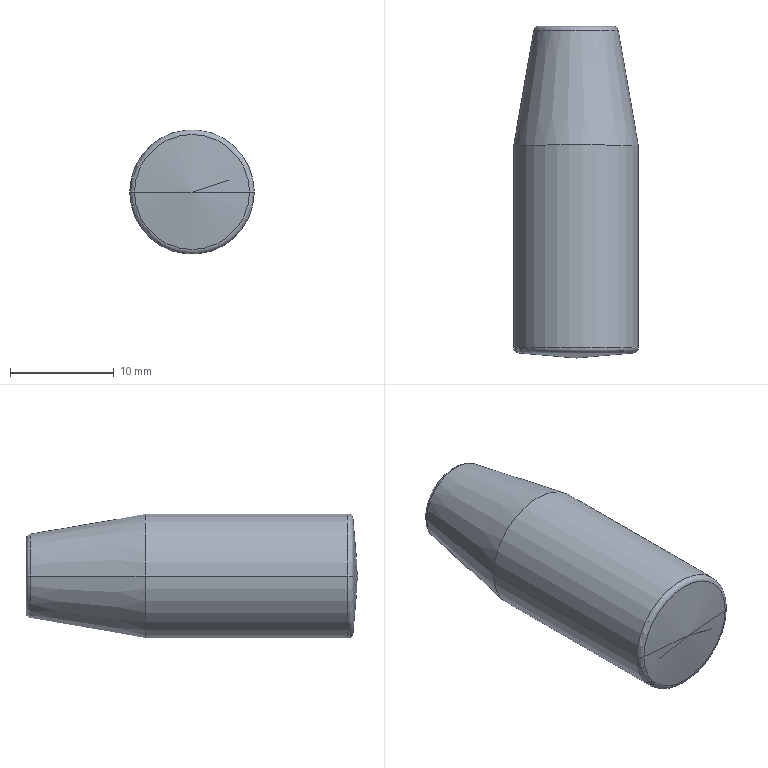Part | NX | 1 solid | 18 faces | box 12 x 32 x 12 mm | volume 2730 mm3 | cylinder 6 | cone 6 | torus 4 | plane 2 | commonest cylinder face diameters 5 x2 6.5 x2 12 x2
STEP:
#1=CARTESIAN_POINT('',(-6.,-19.017,0.));
#2=VERTEX_POINT('',#1);
#3=CARTESIAN_POINT('',(6.,-19.017,0.));
#4=VERTEX_POINT('',#3);
#5=CARTESIAN_POINT('',(0.,-19.017,0.));
#6=DIRECTION('',(0.,-1.,0.));
#7=DIRECTION('',(-1.,0.,0.));
#8=AXIS2_PLACEMENT_3D('',#5,#6,#7);
#9=CIRCLE('',#8,6.);
#10=EDGE_CURVE('',#2,#4,#9,.T.);
#11=ORIENTED_EDGE('',*,*,#10,.F.);
#12=CARTESIAN_POINT('',(-6.,0.5249,0.));
#13=VERTEX_POINT('',#12);
#14=CARTESIAN_POINT('',(-6.,13.6,0.));
#15=DIRECTION('',(0.,-1.,0.));
#16=VECTOR('',#15,1000.);
#17=LINE('',#14,#16);
#18=EDGE_CURVE('',#2,#13,#17,.F.);
#19=ORIENTED_EDGE('',*,*,#18,.T.);
#20=CARTESIAN_POINT('',(6.,0.5249,0.));
#21=VERTEX_POINT('',#20);
#22=CARTESIAN_POINT('',(0.,0.5249,0.));
#23=DIRECTION('',(0.,-1.,0.));
#24=DIRECTION('',(-1.,0.,0.));
#25=AXIS2_PLACEMENT_3D('',#22,#23,#24);
#26=CIRCLE('',#25,6.);
#27=EDGE_CURVE('',#13,#21,#26,.T.);
#28=ORIENTED_EDGE('',*,*,#27,.T.);
#29=CARTESIAN_POINT('',(6.,13.6,0.));
#30=DIRECTION('',(0.,-1.,0.));
#31=VECTOR('',#30,1000.);
#32=LINE('',#29,#31);
#33=EDGE_CURVE('',#4,#21,#32,.F.);
#34=ORIENTED_EDGE('',*,*,#33,.F.);
#35=EDGE_LOOP('',(#11,#19,#28,#34));
#36=FACE_BOUND('',#35,.T.);
#37=CARTESIAN_POINT('',(0.,13.6,0.));
#38=DIRECTION('',(0.,-1.,0.));
#39=DIRECTION('',(-1.,0.,0.));
#40=AXIS2_PLACEMENT_3D('',#37,#38,#39);
#41=CYLINDRICAL_SURFACE('',#40,6.);
#42=ADVANCED_FACE('',(#36),#41,.T.);
#43=ORIENTED_EDGE('',*,*,#10,.T.);
#44=CARTESIAN_POINT('',(5.544,-19.515,0.));
#45=VERTEX_POINT('',#44);
#46=CARTESIAN_POINT('',(5.5,-19.017,0.));
#47=DIRECTION('',(0.,0.,1.));
#48=DIRECTION('',(1.,0.,0.));
#49=AXIS2_PLACEMENT_3D('',#46,#47,#48);
#50=CIRCLE('',#49,0.5);
#51=EDGE_CURVE('',#4,#45,#50,.F.);
#52=ORIENTED_EDGE('',*,*,#51,.T.);
#53=CARTESIAN_POINT('',(-5.544,-19.515,0.));
#54=VERTEX_POINT('',#53);
#55=CARTESIAN_POINT('',(0.,-19.515,0.));
#56=DIRECTION('',(0.,-1.,0.));
#57=DIRECTION('',(-1.,0.,-0.008925));
#58=AXIS2_PLACEMENT_3D('',#55,#56,#57);
#59=CIRCLE('',#58,5.544);
#60=EDGE_CURVE('',#54,#45,#59,.T.);
#61=ORIENTED_EDGE('',*,*,#60,.F.);
#62=CARTESIAN_POINT('',(-5.5,-19.017,0.));
#63=DIRECTION('',(0.,0.,-1.));
#64=DIRECTION('',(-1.,0.,0.));
#65=AXIS2_PLACEMENT_3D('',#62,#63,#64);
#66=CIRCLE('',#65,0.5);
#67=EDGE_CURVE('',#2,#54,#66,.F.);
#68=ORIENTED_EDGE('',*,*,#67,.F.);
#69=EDGE_LOOP('',(#43,#52,#61,#68));
#70=FACE_BOUND('',#69,.T.);
#71=CARTESIAN_POINT('',(0.,-19.017,0.));
#72=DIRECTION('',(0.,-1.,0.));
#73=DIRECTION('',(-1.,0.,0.));
#74=AXIS2_PLACEMENT_3D('',#71,#72,#73);
#75=TOROIDAL_SURFACE('',#74,5.5,0.5);
#76=ADVANCED_FACE('',(#70),#75,.T.);
#77=CARTESIAN_POINT('',(2.5,-9.,0.));
#78=VERTEX_POINT('',#77);
#79=CARTESIAN_POINT('',(-2.5,-9.,0.));
#80=VERTEX_POINT('',#79);
#81=CARTESIAN_POINT('',(0.,-9.,0.));
#82=DIRECTION('',(0.,-1.,0.));
#83=DIRECTION('',(-1.,0.,0.));
#84=AXIS2_PLACEMENT_3D('',#81,#82,#83);
#85=CIRCLE('',#84,2.5);
#86=EDGE_CURVE('',#78,#80,#85,.T.);
#87=ORIENTED_EDGE('',*,*,#86,.F.);
#88=CARTESIAN_POINT('',(0.,-10.502,0.));
#89=VERTEX_POINT('',#88);
#90=CARTESIAN_POINT('',(1.275,-9.736,0.));
#91=DIRECTION('',(0.8572,0.515,0.));
#92=VECTOR('',#91,1000.);
#93=LINE('',#90,#92);
#94=EDGE_CURVE('',#78,#89,#93,.F.);
#95=ORIENTED_EDGE('',*,*,#94,.T.);
#96=CARTESIAN_POINT('',(-1.275,-9.736,0.));
#97=DIRECTION('',(-0.8572,0.515,0.));
#98=VECTOR('',#97,1000.);
#99=LINE('',#96,#98);
#100=EDGE_CURVE('',#80,#89,#99,.F.);
#101=ORIENTED_EDGE('',*,*,#100,.F.);
#102=EDGE_LOOP('',(#87,#95,#101));
#103=FACE_BOUND('',#102,.T.);
#104=CARTESIAN_POINT('',(0.,-9.736,0.));
#105=DIRECTION('',(0.,1.,0.));
#106=DIRECTION('',(1.,0.,0.));
#107=AXIS2_PLACEMENT_3D('',#104,#105,#106);
#108=CONICAL_SURFACE('',#107,1.275,1.03);
#109=ADVANCED_FACE('',(#103),#108,.F.);
#110=CARTESIAN_POINT('',(0.,-20.,0.));
#111=VERTEX_POINT('',#110);
#112=CARTESIAN_POINT('',(-2.827,-19.753,0.));
#113=DIRECTION('',(-0.9962,0.08716,0.));
#114=VECTOR('',#113,1000.);
#115=LINE('',#112,#114);
#116=EDGE_CURVE('',#54,#111,#115,.F.);
#117=ORIENTED_EDGE('',*,*,#116,.F.);
#118=ORIENTED_EDGE('',*,*,#60,.T.);
#119=CARTESIAN_POINT('',(2.827,-19.753,0.));
#120=DIRECTION('',(0.9962,0.08716,0.));
#121=VECTOR('',#120,1000.);
#122=LINE('',#119,#121);
#123=EDGE_CURVE('',#45,#111,#122,.F.);
#124=ORIENTED_EDGE('',*,*,#123,.T.);
#125=EDGE_LOOP('',(#117,#118,#124));
#126=FACE_BOUND('',#125,.T.);
#127=CARTESIAN_POINT('',(0.,-19.753,0.));
#128=DIRECTION('',(0.,1.,0.));
#129=DIRECTION('',(1.,0.,0.));
#130=AXIS2_PLACEMENT_3D('',#127,#128,#129);
#131=CONICAL_SURFACE('',#130,2.827,1.484);
#132=ADVANCED_FACE('',(#126),#131,.T.);
#133=CARTESIAN_POINT('',(4.072,11.586,0.));
#134=VERTEX_POINT('',#133);
#135=CARTESIAN_POINT('',(-4.072,11.586,0.));
#136=VERTEX_POINT('',#135);
#137=CARTESIAN_POINT('',(0.,11.586,0.));
#138=DIRECTION('',(0.,-1.,0.));
#139=DIRECTION('',(0.9999,0.,0.01582));
#140=AXIS2_PLACEMENT_3D('',#137,#138,#139);
#141=CIRCLE('',#140,4.072);
#142=EDGE_CURVE('',#134,#136,#141,.T.);
#143=ORIENTED_EDGE('',*,*,#142,.T.);
#144=CARTESIAN_POINT('',(-5.036,6.055,0.));
#145=DIRECTION('',(-0.1717,-0.9851,0.));
#146=VECTOR('',#145,1000.);
#147=LINE('',#144,#146);
#148=EDGE_CURVE('',#13,#136,#147,.F.);
#149=ORIENTED_EDGE('',*,*,#148,.F.);
#150=CARTESIAN_POINT('',(0.,0.5249,0.));
#151=DIRECTION('',(0.,-1.,0.));
#152=DIRECTION('',(-1.,0.,0.));
#153=AXIS2_PLACEMENT_3D('',#150,#151,#152);
#154=CIRCLE('',#153,6.);
#155=EDGE_CURVE('',#21,#13,#154,.T.);
#156=ORIENTED_EDGE('',*,*,#155,.F.);
#157=CARTESIAN_POINT('',(5.036,6.055,0.));
#158=DIRECTION('',(0.1717,-0.9851,0.));
#159=VECTOR('',#158,1000.);
#160=LINE('',#157,#159);
#161=EDGE_CURVE('',#21,#134,#160,.F.);
#162=ORIENTED_EDGE('',*,*,#161,.T.);
#163=EDGE_LOOP('',(#143,#149,#156,#162));
#164=FACE_BOUND('',#163,.T.);
#165=CARTESIAN_POINT('',(0.,6.055,0.));
#166=DIRECTION('',(0.,-1.,0.));
#167=DIRECTION('',(-1.,0.,0.));
#168=AXIS2_PLACEMENT_3D('',#165,#166,#167);
#169=CONICAL_SURFACE('',#168,5.036,0.1726);
#170=ADVANCED_FACE('',(#164),#169,.T.);
#171=ORIENTED_EDGE('',*,*,#142,.F.);
#172=CARTESIAN_POINT('',(3.58,12.,0.));
#173=VERTEX_POINT('',#172);
#174=CARTESIAN_POINT('',(3.58,11.5,0.));
#175=DIRECTION('',(0.,0.,1.));
#176=DIRECTION('',(1.,0.,0.));
#177=AXIS2_PLACEMENT_3D('',#174,#175,#176);
#178=CIRCLE('',#177,0.5);
#179=EDGE_CURVE('',#173,#134,#178,.F.);
#180=ORIENTED_EDGE('',*,*,#179,.F.);
#181=CARTESIAN_POINT('',(-3.58,12.,0.));
#182=VERTEX_POINT('',#181);
#183=CARTESIAN_POINT('',(0.,12.,0.));
#184=DIRECTION('',(0.,-1.,0.));
#185=DIRECTION('',(0.9999,0.,0.01582));
#186=AXIS2_PLACEMENT_3D('',#183,#184,#185);
#187=CIRCLE('',#186,3.58);
#188=EDGE_CURVE('',#173,#182,#187,.T.);
#189=ORIENTED_EDGE('',*,*,#188,.T.);
#190=CARTESIAN_POINT('',(-3.58,11.5,0.));
#191=DIRECTION('',(0.,0.,-1.));
#192=DIRECTION('',(-1.,0.,0.));
#193=AXIS2_PLACEMENT_3D('',#190,#191,#192);
#194=CIRCLE('',#193,0.5);
#195=EDGE_CURVE('',#182,#136,#194,.F.);
#196=ORIENTED_EDGE('',*,*,#195,.T.);
#197=EDGE_LOOP('',(#171,#180,#189,#196));
#198=FACE_BOUND('',#197,.T.);
#199=CARTESIAN_POINT('',(0.,11.5,0.));
#200=DIRECTION('',(0.,-1.,0.));
#201=DIRECTION('',(-1.,0.,0.));
#202=AXIS2_PLACEMENT_3D('',#199,#200,#201);
#203=TOROIDAL_SURFACE('',#202,3.58,0.5);
#204=ADVANCED_FACE('',(#198),#203,.T.);
#205=ORIENTED_EDGE('',*,*,#188,.F.);
#206=CARTESIAN_POINT('',(0.,12.,0.));
#207=DIRECTION('',(0.,-1.,0.));
#208=DIRECTION('',(0.9999,0.,0.01582));
#209=AXIS2_PLACEMENT_3D('',#206,#207,#208);
#210=CIRCLE('',#209,3.58);
#211=EDGE_CURVE('',#182,#173,#210,.T.);
#212=ORIENTED_EDGE('',*,*,#211,.F.);
#213=EDGE_LOOP('',(#205,#212));
#214=FACE_BOUND('',#213,.T.);
#215=CARTESIAN_POINT('',(3.25,12.,0.));
#216=VERTEX_POINT('',#215);
#217=CARTESIAN_POINT('',(-3.25,12.,0.));
#218=VERTEX_POINT('',#217);
#219=CARTESIAN_POINT('',(0.,12.,0.));
#220=DIRECTION('',(0.,1.,0.));
#221=DIRECTION('',(1.,0.,0.));
#222=AXIS2_PLACEMENT_3D('',#219,#220,#221);
#223=CIRCLE('',#222,3.25);
#224=EDGE_CURVE('',#216,#218,#223,.T.);
#225=ORIENTED_EDGE('',*,*,#224,.F.);
#226=CARTESIAN_POINT('',(0.,12.,0.));
#227=DIRECTION('',(0.,1.,0.));
#228=DIRECTION('',(1.,0.,0.));
#229=AXIS2_PLACEMENT_3D('',#226,#227,#228);
#230=CIRCLE('',#229,3.25);
#231=EDGE_CURVE('',#218,#216,#230,.T.);
#232=ORIENTED_EDGE('',*,*,#231,.F.);
#233=EDGE_LOOP('',(#225,#232));
#234=FACE_BOUND('',#233,.T.);
#235=CARTESIAN_POINT('',(0.,12.,0.));
#236=DIRECTION('',(0.,-1.,0.));
#237=DIRECTION('',(0.,0.,-1.));
#238=AXIS2_PLACEMENT_3D('',#235,#236,#237);
#239=PLANE('',#238);
#240=ADVANCED_FACE('',(#214,#234),#239,.F.);
#241=CARTESIAN_POINT('',(3.25,9.,0.));
#242=VERTEX_POINT('',#241);
#243=CARTESIAN_POINT('',(-3.25,9.,0.));
#244=VERTEX_POINT('',#243);
#245=CARTESIAN_POINT('',(0.,9.,0.));
#246=DIRECTION('',(0.,-1.,0.));
#247=DIRECTION('',(-1.,0.,0.));
#248=AXIS2_PLACEMENT_3D('',#245,#246,#247);
#249=CIRCLE('',#248,3.25);
#250=EDGE_CURVE('',#242,#244,#249,.T.);
#251=ORIENTED_EDGE('',*,*,#250,.F.);
#252=CARTESIAN_POINT('',(0.,9.,0.));
#253=DIRECTION('',(0.,-1.,0.));
#254=DIRECTION('',(-1.,0.,0.));
#255=AXIS2_PLACEMENT_3D('',#252,#253,#254);
#256=CIRCLE('',#255,3.25);
#257=EDGE_CURVE('',#244,#242,#256,.T.);
#258=ORIENTED_EDGE('',*,*,#257,.F.);
#259=EDGE_LOOP('',(#251,#258));
#260=FACE_BOUND('',#259,.T.);
#261=CARTESIAN_POINT('',(-2.5,9.,0.));
#262=VERTEX_POINT('',#261);
#263=CARTESIAN_POINT('',(2.5,9.,0.));
#264=VERTEX_POINT('',#263);
#265=CARTESIAN_POINT('',(0.,9.,0.));
#266=DIRECTION('',(0.,1.,0.));
#267=DIRECTION('',(-1.,0.,0.));
#268=AXIS2_PLACEMENT_3D('',#265,#266,#267);
#269=CIRCLE('',#268,2.5);
#270=EDGE_CURVE('',#262,#264,#269,.T.);
#271=ORIENTED_EDGE('',*,*,#270,.F.);
#272=CARTESIAN_POINT('',(0.,9.,0.));
#273=DIRECTION('',(0.,1.,0.));
#274=DIRECTION('',(-1.,0.,0.));
#275=AXIS2_PLACEMENT_3D('',#272,#273,#274);
#276=CIRCLE('',#275,2.5);
#277=EDGE_CURVE('',#264,#262,#276,.T.);
#278=ORIENTED_EDGE('',*,*,#277,.F.);
#279=EDGE_LOOP('',(#271,#278));
#280=FACE_BOUND('',#279,.T.);
#281=CARTESIAN_POINT('',(0.,9.,0.));
#282=DIRECTION('',(0.,-1.,0.));
#283=DIRECTION('',(0.,0.,-1.));
#284=AXIS2_PLACEMENT_3D('',#281,#282,#283);
#285=PLANE('',#284);
#286=ADVANCED_FACE('',(#260,#280),#285,.F.);
#287=ORIENTED_EDGE('',*,*,#270,.T.);
#288=CARTESIAN_POINT('',(2.5,-11.477,0.));
#289=DIRECTION('',(0.,1.,0.));
#290=VECTOR('',#289,1000.);
#291=LINE('',#288,#290);
#292=EDGE_CURVE('',#78,#264,#291,.T.);
#293=ORIENTED_EDGE('',*,*,#292,.F.);
#294=ORIENTED_EDGE('',*,*,#86,.T.);
#295=CARTESIAN_POINT('',(-2.5,-11.477,0.));
#296=DIRECTION('',(0.,1.,0.));
#297=VECTOR('',#296,1000.);
#298=LINE('',#295,#297);
#299=EDGE_CURVE('',#80,#262,#298,.T.);
#300=ORIENTED_EDGE('',*,*,#299,.T.);
#301=EDGE_LOOP('',(#287,#293,#294,#300));
#302=FACE_BOUND('',#301,.T.);
#303=CARTESIAN_POINT('',(0.,-11.477,0.));
#304=DIRECTION('',(0.,1.,0.));
#305=DIRECTION('',(1.,0.,0.));
#306=AXIS2_PLACEMENT_3D('',#303,#304,#305);
#307=CYLINDRICAL_SURFACE('',#306,2.5);
#308=ADVANCED_FACE('',(#302),#307,.F.);
#309=ORIENTED_EDGE('',*,*,#250,.T.);
#310=CARTESIAN_POINT('',(-3.25,12.,0.));
#311=DIRECTION('',(0.,-1.,0.));
#312=VECTOR('',#311,1000.);
#313=LINE('',#310,#312);
#314=EDGE_CURVE('',#244,#218,#313,.F.);
#315=ORIENTED_EDGE('',*,*,#314,.T.);
#316=ORIENTED_EDGE('',*,*,#231,.T.);
#317=CARTESIAN_POINT('',(3.25,12.,0.));
#318=DIRECTION('',(0.,-1.,0.));
#319=VECTOR('',#318,1000.);
#320=LINE('',#317,#319);
#321=EDGE_CURVE('',#242,#216,#320,.F.);
#322=ORIENTED_EDGE('',*,*,#321,.F.);
#323=EDGE_LOOP('',(#309,#315,#316,#322));
#324=FACE_BOUND('',#323,.T.);
#325=CARTESIAN_POINT('',(0.,12.,0.));
#326=DIRECTION('',(0.,-1.,0.));
#327=DIRECTION('',(1.,0.,0.));
#328=AXIS2_PLACEMENT_3D('',#325,#326,#327);
#329=CYLINDRICAL_SURFACE('',#328,3.25);
#330=ADVANCED_FACE('',(#324),#329,.F.);
#331=ORIENTED_EDGE('',*,*,#292,.T.);
#332=ORIENTED_EDGE('',*,*,#277,.T.);
#333=ORIENTED_EDGE('',*,*,#299,.F.);
#334=CARTESIAN_POINT('',(0.,-9.,0.));
#335=DIRECTION('',(0.,-1.,0.));
#336=DIRECTION('',(-1.,0.,0.));
#337=AXIS2_PLACEMENT_3D('',#334,#335,#336);
#338=CIRCLE('',#337,2.5);
#339=EDGE_CURVE('',#80,#78,#338,.T.);
#340=ORIENTED_EDGE('',*,*,#339,.T.);
#341=EDGE_LOOP('',(#331,#332,#333,#340));
#342=FACE_BOUND('',#341,.T.);
#343=CARTESIAN_POINT('',(0.,-11.477,0.));
#344=DIRECTION('',(0.,1.,0.));
#345=DIRECTION('',(1.,0.,0.));
#346=AXIS2_PLACEMENT_3D('',#343,#344,#345);
#347=CYLINDRICAL_SURFACE('',#346,2.5);
#348=ADVANCED_FACE('',(#342),#347,.F.);
#349=ORIENTED_EDGE('',*,*,#116,.T.);
#350=ORIENTED_EDGE('',*,*,#123,.F.);
#351=CARTESIAN_POINT('',(0.,-19.515,0.));
#352=DIRECTION('',(0.,-1.,0.));
#353=DIRECTION('',(-1.,0.,-0.008925));
#354=AXIS2_PLACEMENT_3D('',#351,#352,#353);
#355=CIRCLE('',#354,5.544);
#356=EDGE_CURVE('',#45,#54,#355,.T.);
#357=ORIENTED_EDGE('',*,*,#356,.T.);
#358=EDGE_LOOP('',(#349,#350,#357));
#359=FACE_BOUND('',#358,.T.);
#360=CARTESIAN_POINT('',(0.,-19.753,0.));
#361=DIRECTION('',(0.,1.,0.));
#362=DIRECTION('',(1.,0.,0.));
#363=AXIS2_PLACEMENT_3D('',#360,#361,#362);
#364=CONICAL_SURFACE('',#363,2.827,1.484);
#365=ADVANCED_FACE('',(#359),#364,.T.);
#366=ORIENTED_EDGE('',*,*,#100,.T.);
#367=ORIENTED_EDGE('',*,*,#94,.F.);
#368=ORIENTED_EDGE('',*,*,#339,.F.);
#369=EDGE_LOOP('',(#366,#367,#368));
#370=FACE_BOUND('',#369,.T.);
#371=CARTESIAN_POINT('',(0.,-9.736,0.));
#372=DIRECTION('',(0.,1.,0.));
#373=DIRECTION('',(1.,0.,0.));
#374=AXIS2_PLACEMENT_3D('',#371,#372,#373);
#375=CONICAL_SURFACE('',#374,1.275,1.03);
#376=ADVANCED_FACE('',(#370),#375,.F.);
#377=ORIENTED_EDGE('',*,*,#224,.T.);
#378=ORIENTED_EDGE('',*,*,#314,.F.);
#379=ORIENTED_EDGE('',*,*,#257,.T.);
#380=ORIENTED_EDGE('',*,*,#321,.T.);
#381=EDGE_LOOP('',(#377,#378,#379,#380));
#382=FACE_BOUND('',#381,.T.);
#383=CARTESIAN_POINT('',(0.,12.,0.));
#384=DIRECTION('',(0.,-1.,0.));
#385=DIRECTION('',(1.,0.,0.));
#386=AXIS2_PLACEMENT_3D('',#383,#384,#385);
#387=CYLINDRICAL_SURFACE('',#386,3.25);
#388=ADVANCED_FACE('',(#382),#387,.F.);
#389=ORIENTED_EDGE('',*,*,#27,.F.);
#390=ORIENTED_EDGE('',*,*,#148,.T.);
#391=CARTESIAN_POINT('',(0.,11.586,0.));
#392=DIRECTION('',(0.,-1.,0.));
#393=DIRECTION('',(0.9999,0.,0.01582));
#394=AXIS2_PLACEMENT_3D('',#391,#392,#393);
#395=CIRCLE('',#394,4.072);
#396=EDGE_CURVE('',#136,#134,#395,.T.);
#397=ORIENTED_EDGE('',*,*,#396,.T.);
#398=ORIENTED_EDGE('',*,*,#161,.F.);
#399=EDGE_LOOP('',(#389,#390,#397,#398));
#400=FACE_BOUND('',#399,.T.);
#401=CARTESIAN_POINT('',(0.,6.055,0.));
#402=DIRECTION('',(0.,-1.,0.));
#403=DIRECTION('',(-1.,0.,0.));
#404=AXIS2_PLACEMENT_3D('',#401,#402,#403);
#405=CONICAL_SURFACE('',#404,5.036,0.1726);
#406=ADVANCED_FACE('',(#400),#405,.T.);
#407=ORIENTED_EDGE('',*,*,#18,.F.);
#408=CARTESIAN_POINT('',(0.,-19.017,0.));
#409=DIRECTION('',(0.,-1.,0.));
#410=DIRECTION('',(-1.,0.,0.));
#411=AXIS2_PLACEMENT_3D('',#408,#409,#410);
#412=CIRCLE('',#411,6.);
#413=EDGE_CURVE('',#4,#2,#412,.T.);
#414=ORIENTED_EDGE('',*,*,#413,.F.);
#415=ORIENTED_EDGE('',*,*,#33,.T.);
#416=ORIENTED_EDGE('',*,*,#155,.T.);
#417=EDGE_LOOP('',(#407,#414,#415,#416));
#418=FACE_BOUND('',#417,.T.);
#419=CARTESIAN_POINT('',(0.,13.6,0.));
#420=DIRECTION('',(0.,-1.,0.));
#421=DIRECTION('',(-1.,0.,0.));
#422=AXIS2_PLACEMENT_3D('',#419,#420,#421);
#423=CYLINDRICAL_SURFACE('',#422,6.);
#424=ADVANCED_FACE('',(#418),#423,.T.);
#425=ORIENTED_EDGE('',*,*,#195,.F.);
#426=ORIENTED_EDGE('',*,*,#211,.T.);
#427=ORIENTED_EDGE('',*,*,#179,.T.);
#428=ORIENTED_EDGE('',*,*,#396,.F.);
#429=EDGE_LOOP('',(#425,#426,#427,#428));
#430=FACE_BOUND('',#429,.T.);
#431=CARTESIAN_POINT('',(0.,11.5,0.));
#432=DIRECTION('',(0.,-1.,0.));
#433=DIRECTION('',(-1.,0.,0.));
#434=AXIS2_PLACEMENT_3D('',#431,#432,#433);
#435=TOROIDAL_SURFACE('',#434,3.58,0.5);
#436=ADVANCED_FACE('',(#430),#435,.T.);
#437=ORIENTED_EDGE('',*,*,#67,.T.);
#438=ORIENTED_EDGE('',*,*,#356,.F.);
#439=ORIENTED_EDGE('',*,*,#51,.F.);
#440=ORIENTED_EDGE('',*,*,#413,.T.);
#441=EDGE_LOOP('',(#437,#438,#439,#440));
#442=FACE_BOUND('',#441,.T.);
#443=CARTESIAN_POINT('',(0.,-19.017,0.));
#444=DIRECTION('',(0.,-1.,0.));
#445=DIRECTION('',(-1.,0.,0.));
#446=AXIS2_PLACEMENT_3D('',#443,#444,#445);
#447=TOROIDAL_SURFACE('',#446,5.5,0.5);
#448=ADVANCED_FACE('',(#442),#447,.T.);
#449=CLOSED_SHELL('',(#42,#76,#109,#132,#170,#204,#240,#286,#308,#330,#348,#365,#376,#388,#406,#424,#436,#448));
#450=MANIFOLD_SOLID_BREP('',#449);
#451=(LENGTH_UNIT()NAMED_UNIT(*)SI_UNIT(.MILLI.,.METRE.));
#452=UNCERTAINTY_MEASURE_WITH_UNIT(LENGTH_MEASURE(0.00001),#451,'','');
#453=(NAMED_UNIT(*)PLANE_ANGLE_UNIT()SI_UNIT($,.RADIAN.));
#454=(NAMED_UNIT(*)SI_UNIT($,.STERADIAN.)SOLID_ANGLE_UNIT());
#455=(GEOMETRIC_REPRESENTATION_CONTEXT(3)GLOBAL_UNCERTAINTY_ASSIGNED_CONTEXT((#452))GLOBAL_UNIT_ASSIGNED_CONTEXT((#451,#453,#454))REPRESENTATION_CONTEXT('',''));
#456=ADVANCED_BREP_SHAPE_REPRESENTATION('',(#450),#455);